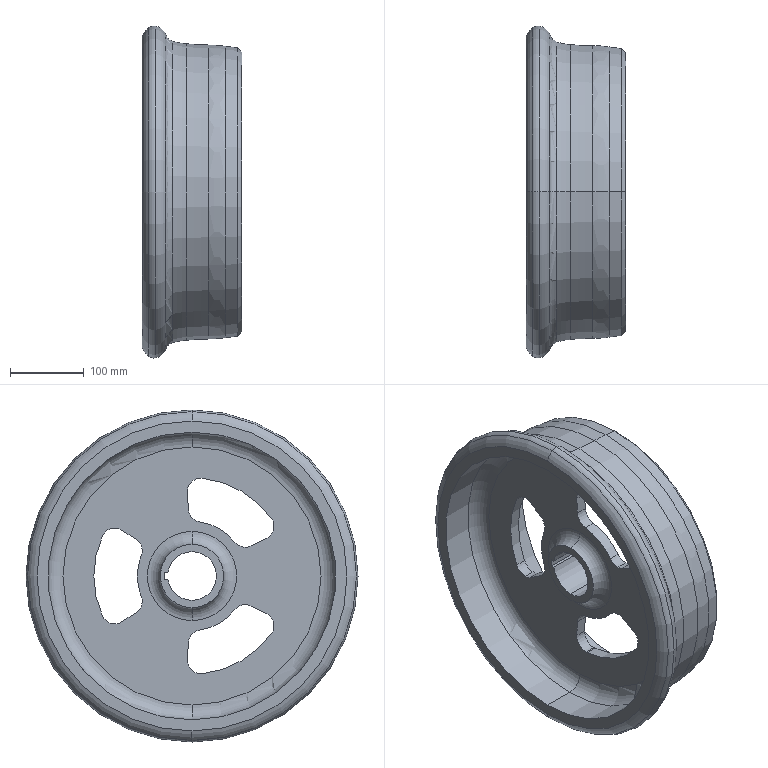Part | STEP file | LM wheel | 1 solid | 69 faces | box 135 x 449.742 x 449.742 mm | volume 4161570 mm3 | cylinder 28 | torus 22 | plane 15 | cone 4 | commonest cylinder face diameters 36 x15 66 x3 148 x3 266 x3 369.276 x2 389.742 x2